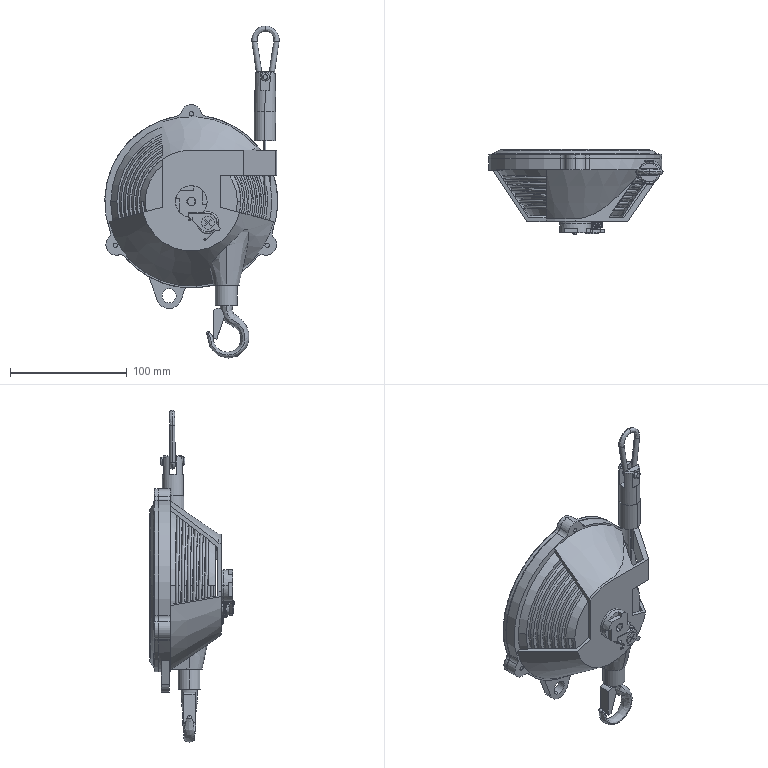Part | STEP file | EW-3 | 10 solids | 393 faces | box 149.256 x 72.65 x 284.25 mm | volume 626000 mm3 | plane 162 | cylinder 119 | spline 68 | cone 43 | sphere 1 | commonest cylinder face diameters 10 x14 1.5 x10 18 x10 7.5 x7 15 x7 148 x7